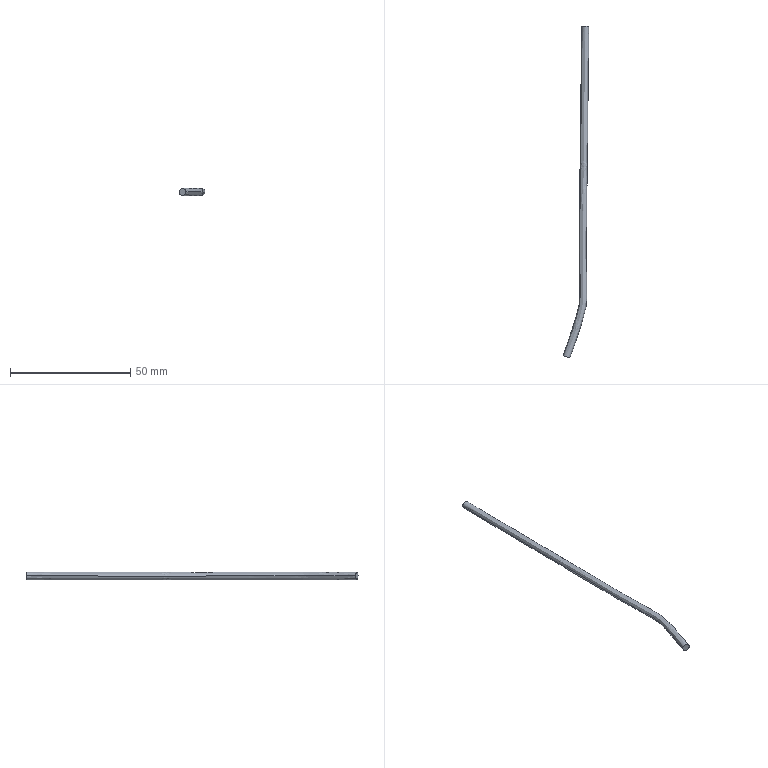Part | NX | features BREP 1 | 1 solid | 4 faces | box 10.731 x 138.267 x 3 mm | volume 970.254 mm3 | plane 2 | spline 2
STEP:
#1=CARTESIAN_POINT('',(62.397,243.449,217.465));
#2=VERTEX_POINT('',#1);
#3=CARTESIAN_POINT('',(65.397,243.411,217.465));
#4=VERTEX_POINT('',#3);
#5=CARTESIAN_POINT('',(62.397,243.449,217.465));
#6=CARTESIAN_POINT('',(62.397,243.449,217.111));
#7=CARTESIAN_POINT('',(62.665,243.445,216.338));
#8=CARTESIAN_POINT('',(63.897,243.43,215.778));
#9=CARTESIAN_POINT('',(65.129,243.415,216.338));
#10=CARTESIAN_POINT('',(65.397,243.411,217.111));
#11=CARTESIAN_POINT('',(65.397,243.411,217.465));
#12=B_SPLINE_CURVE_WITH_KNOTS('',3,(#5,#6,#7,#8,#9,#10,#11),.UNSPECIFIED.,.F.,.F.,(4,1,1,1,4),(0.,0.25,0.5,0.75,1.),.UNSPECIFIED.);
#13=EDGE_CURVE('',#2,#4,#12,.T.);
#14=ORIENTED_EDGE('',*,*,#13,.F.);
#15=CARTESIAN_POINT('',(65.397,243.411,217.465));
#16=CARTESIAN_POINT('',(65.397,243.411,217.819));
#17=CARTESIAN_POINT('',(65.129,243.415,218.592));
#18=CARTESIAN_POINT('',(63.897,243.43,219.152));
#19=CARTESIAN_POINT('',(62.665,243.445,218.592));
#20=CARTESIAN_POINT('',(62.397,243.449,217.819));
#21=CARTESIAN_POINT('',(62.397,243.449,217.465));
#22=B_SPLINE_CURVE_WITH_KNOTS('',3,(#15,#16,#17,#18,#19,#20,#21),.UNSPECIFIED.,.F.,.F.,(4,1,1,1,4),(0.,0.25,0.5,0.75,1.),.UNSPECIFIED.);
#23=EDGE_CURVE('',#4,#2,#22,.T.);
#24=ORIENTED_EDGE('',*,*,#23,.F.);
#25=EDGE_LOOP('',(#14,#24));
#26=FACE_BOUND('',#25,.T.);
#27=CARTESIAN_POINT('',(63.897,243.43,217.465));
#28=DIRECTION('',(0.01249,0.9999,0.000000006));
#29=DIRECTION('',(-0.000000489,0.,1.));
#30=AXIS2_PLACEMENT_3D('',#27,#28,#29);
#31=PLANE('',#30);
#32=ADVANCED_FACE('',(#26),#31,.T.);
#33=CARTESIAN_POINT('',(54.666,106.175,217.465));
#34=VERTEX_POINT('',#33);
#35=CARTESIAN_POINT('',(54.666,106.175,217.465));
#36=CARTESIAN_POINT('',(54.959,107.01,217.465));
#37=CARTESIAN_POINT('',(55.542,108.723,217.465));
#38=CARTESIAN_POINT('',(56.487,111.418,217.465));
#39=CARTESIAN_POINT('',(57.437,114.09,217.465));
#40=CARTESIAN_POINT('',(58.24,116.429,217.465));
#41=CARTESIAN_POINT('',(58.924,118.557,217.465));
#42=CARTESIAN_POINT('',(59.672,121.018,217.465));
#43=CARTESIAN_POINT('',(60.34,123.36,217.465));
#44=CARTESIAN_POINT('',(60.967,125.706,217.465));
#45=CARTESIAN_POINT('',(61.279,127.056,217.465));
#46=CARTESIAN_POINT('',(61.434,128.236,217.465));
#47=CARTESIAN_POINT('',(61.516,129.688,217.465));
#48=CARTESIAN_POINT('',(61.555,131.384,217.465));
#49=CARTESIAN_POINT('',(61.564,133.089,217.465));
#50=CARTESIAN_POINT('',(61.559,134.799,217.465));
#51=CARTESIAN_POINT('',(61.543,136.834,217.465));
#52=CARTESIAN_POINT('',(61.518,138.999,217.465));
#53=CARTESIAN_POINT('',(61.487,141.254,217.465));
#54=CARTESIAN_POINT('',(61.457,143.133,217.465));
#55=CARTESIAN_POINT('',(61.431,144.64,217.465));
#56=CARTESIAN_POINT('',(61.415,145.483,217.465));
#57=CARTESIAN_POINT('',(61.404,146.066,217.465));
#58=CARTESIAN_POINT('',(61.391,146.692,217.465));
#59=CARTESIAN_POINT('',(61.365,147.969,217.465));
#60=CARTESIAN_POINT('',(61.335,149.222,217.465));
#61=CARTESIAN_POINT('',(61.318,149.829,217.465));
#62=CARTESIAN_POINT('',(61.309,150.1,217.465));
#63=CARTESIAN_POINT('',(61.304,150.384,217.465));
#64=CARTESIAN_POINT('',(61.304,150.773,217.465));
#65=CARTESIAN_POINT('',(61.306,151.152,217.465));
#66=CARTESIAN_POINT('',(61.311,151.792,217.465));
#67=CARTESIAN_POINT('',(61.321,152.752,217.465));
#68=CARTESIAN_POINT('',(61.336,154.044,217.465));
#69=CARTESIAN_POINT('',(61.35,155.324,217.465));
#70=CARTESIAN_POINT('',(61.403,159.651,217.465));
#71=CARTESIAN_POINT('',(61.499,167.097,217.465));
#72=CARTESIAN_POINT('',(61.64,178.866,217.465));
#73=CARTESIAN_POINT('',(61.75,188.661,217.465));
#74=CARTESIAN_POINT('',(61.833,195.881,217.465));
#75=CARTESIAN_POINT('',(61.915,202.983,217.465));
#76=CARTESIAN_POINT('',(62.024,211.946,217.465));
#77=CARTESIAN_POINT('',(62.15,222.241,217.465));
#78=CARTESIAN_POINT('',(62.269,232.536,217.465));
#79=CARTESIAN_POINT('',(62.351,239.794,217.465));
#80=CARTESIAN_POINT('',(62.397,243.449,217.465));
#81=B_SPLINE_CURVE_WITH_KNOTS('',3,(#35,#36,#37,#38,#39,#40,#41,#42,#43,#44,#45,#46,#47,#48,#49,#50,#51,#52,#53,#54,#55,#56,#57,#58,#59,#60,#61,#62,#63,#64,#65,#66,#67,#68,#69,#70,#71,#72,#73,#74,#75,#76,#77,#78,#79,#80),.UNSPECIFIED.,.F.,.F.,(4,1,1,1,1,1,1,1,1,1,1,1,1,1,1,1,1,1,1,1,1,1,1,1,1,1,1,1,1,1,1,1,1,1,1,1,1,1,1,1,1,1,1,4),(0.,0.01988,0.03976,0.05964,0.07952,0.09481,0.1101,0.1407,0.1517,0.1628,0.1724,0.1821,0.1966,0.2112,0.2257,0.2402,0.2569,0.2736,0.2903,0.2987,0.307,0.3092,0.3114,0.3158,0.3201,0.3223,0.3245,0.3262,0.3278,0.3295,0.3311,0.3413,0.3515,0.3616,0.3718,0.4479,0.5239,0.6,0.638,0.676,0.757,0.838,0.919,1.),.UNSPECIFIED.);
#82=EDGE_CURVE('',#34,#2,#81,.T.);
#83=ORIENTED_EDGE('',*,*,#82,.T.);
#84=ORIENTED_EDGE('',*,*,#13,.T.);
#85=CARTESIAN_POINT('',(57.496,105.181,217.465));
#86=VERTEX_POINT('',#85);
#87=CARTESIAN_POINT('',(57.496,105.181,217.465));
#88=CARTESIAN_POINT('',(57.797,106.038,217.465));
#89=CARTESIAN_POINT('',(58.377,107.742,217.465));
#90=CARTESIAN_POINT('',(59.312,110.41,217.465));
#91=CARTESIAN_POINT('',(60.267,113.093,217.465));
#92=CARTESIAN_POINT('',(61.086,115.481,217.465));
#93=CARTESIAN_POINT('',(61.788,117.663,217.465));
#94=CARTESIAN_POINT('',(62.554,120.187,217.465));
#95=CARTESIAN_POINT('',(63.229,122.55,217.465));
#96=CARTESIAN_POINT('',(63.871,124.952,217.465));
#97=CARTESIAN_POINT('',(64.23,126.487,217.465));
#98=CARTESIAN_POINT('',(64.427,127.985,217.465));
#99=CARTESIAN_POINT('',(64.515,129.591,217.465));
#100=CARTESIAN_POINT('',(64.555,131.345,217.465));
#101=CARTESIAN_POINT('',(64.563,133.083,217.465));
#102=CARTESIAN_POINT('',(64.559,134.816,217.465));
#103=CARTESIAN_POINT('',(64.543,136.865,217.465));
#104=CARTESIAN_POINT('',(64.518,139.037,217.465));
#105=CARTESIAN_POINT('',(64.486,141.298,217.465));
#106=CARTESIAN_POINT('',(64.457,143.182,217.465));
#107=CARTESIAN_POINT('',(64.43,144.694,217.465));
#108=CARTESIAN_POINT('',(64.415,145.54,217.465));
#109=CARTESIAN_POINT('',(64.403,146.124,217.465));
#110=CARTESIAN_POINT('',(64.391,146.741,217.465));
#111=CARTESIAN_POINT('',(64.365,147.996,217.465));
#112=CARTESIAN_POINT('',(64.334,149.272,217.465));
#113=CARTESIAN_POINT('',(64.316,149.911,217.465));
#114=CARTESIAN_POINT('',(64.308,150.184,217.465));
#115=CARTESIAN_POINT('',(64.304,150.421,217.465));
#116=CARTESIAN_POINT('',(64.304,150.771,217.465));
#117=CARTESIAN_POINT('',(64.306,151.131,217.465));
#118=CARTESIAN_POINT('',(64.311,151.763,217.465));
#119=CARTESIAN_POINT('',(64.321,152.722,217.465));
#120=CARTESIAN_POINT('',(64.335,154.013,217.465));
#121=CARTESIAN_POINT('',(64.35,155.289,217.465));
#122=CARTESIAN_POINT('',(64.402,159.612,217.465));
#123=CARTESIAN_POINT('',(64.499,167.062,217.465));
#124=CARTESIAN_POINT('',(64.64,178.833,217.465));
#125=CARTESIAN_POINT('',(64.75,188.628,217.465));
#126=CARTESIAN_POINT('',(64.832,195.846,217.465));
#127=CARTESIAN_POINT('',(64.915,202.948,217.465));
#128=CARTESIAN_POINT('',(65.024,211.91,217.465));
#129=CARTESIAN_POINT('',(65.15,222.206,217.465));
#130=CARTESIAN_POINT('',(65.269,232.504,217.465));
#131=CARTESIAN_POINT('',(65.351,239.759,217.465));
#132=CARTESIAN_POINT('',(65.397,243.411,217.465));
#133=B_SPLINE_CURVE_WITH_KNOTS('',3,(#87,#88,#89,#90,#91,#92,#93,#94,#95,#96,#97,#98,#99,#100,#101,#102,#103,#104,#105,#106,#107,#108,#109,#110,#111,#112,#113,#114,#115,#116,#117,#118,#119,#120,#121,#122,#123,#124,#125,#126,#127,#128,#129,#130,#131,#132),.UNSPECIFIED.,.F.,.F.,(4,1,1,1,1,1,1,1,1,1,1,1,1,1,1,1,1,1,1,1,1,1,1,1,1,1,1,1,1,1,1,1,1,1,1,1,1,1,1,1,1,1,1,4),(0.,0.01988,0.03976,0.05964,0.07952,0.09481,0.1101,0.1407,0.1517,0.1628,0.1724,0.1821,0.1966,0.2112,0.2257,0.2402,0.2569,0.2736,0.2903,0.2987,0.307,0.3092,0.3114,0.3158,0.3201,0.3223,0.3245,0.3262,0.3278,0.3295,0.3311,0.3413,0.3515,0.3616,0.3718,0.4479,0.5239,0.6,0.638,0.676,0.757,0.838,0.919,1.),.UNSPECIFIED.);
#134=EDGE_CURVE('',#86,#4,#133,.T.);
#135=ORIENTED_EDGE('',*,*,#134,.F.);
#136=CARTESIAN_POINT('',(54.666,106.175,217.465));
#137=CARTESIAN_POINT('',(54.666,106.175,217.111));
#138=CARTESIAN_POINT('',(54.919,106.086,216.338));
#139=CARTESIAN_POINT('',(56.081,105.678,215.778));
#140=CARTESIAN_POINT('',(57.243,105.27,216.338));
#141=CARTESIAN_POINT('',(57.496,105.181,217.111));
#142=CARTESIAN_POINT('',(57.496,105.181,217.465));
#143=B_SPLINE_CURVE_WITH_KNOTS('',3,(#136,#137,#138,#139,#140,#141,#142),.UNSPECIFIED.,.F.,.F.,(4,1,1,1,4),(0.,0.25,0.5,0.75,1.),.UNSPECIFIED.);
#144=EDGE_CURVE('',#34,#86,#143,.T.);
#145=ORIENTED_EDGE('',*,*,#144,.F.);
#146=EDGE_LOOP('',(#83,#84,#135,#145));
#147=FACE_BOUND('',#146,.T.);
#148=CARTESIAN_POINT('',(65.397,243.411,217.465));
#149=CARTESIAN_POINT('',(65.397,243.411,217.111));
#150=CARTESIAN_POINT('',(65.129,243.415,216.338));
#151=CARTESIAN_POINT('',(63.897,243.43,215.778));
#152=CARTESIAN_POINT('',(62.665,243.445,216.338));
#153=CARTESIAN_POINT('',(62.397,243.449,217.111));
#154=CARTESIAN_POINT('',(62.397,243.449,217.465));
#155=CARTESIAN_POINT('',(65.351,239.759,217.465));
#156=CARTESIAN_POINT('',(65.351,239.759,217.111));
#157=CARTESIAN_POINT('',(65.083,239.763,216.338));
#158=CARTESIAN_POINT('',(63.851,239.777,215.778));
#159=CARTESIAN_POINT('',(62.62,239.791,216.338));
#160=CARTESIAN_POINT('',(62.351,239.794,217.111));
#161=CARTESIAN_POINT('',(62.351,239.794,217.465));
#162=CARTESIAN_POINT('',(65.269,232.504,217.465));
#163=CARTESIAN_POINT('',(65.269,232.504,217.111));
#164=CARTESIAN_POINT('',(65.001,232.506,216.338));
#165=CARTESIAN_POINT('',(63.769,232.52,215.778));
#166=CARTESIAN_POINT('',(62.537,232.533,216.338));
#167=CARTESIAN_POINT('',(62.269,232.536,217.111));
#168=CARTESIAN_POINT('',(62.269,232.536,217.465));
#169=CARTESIAN_POINT('',(65.15,222.206,217.465));
#170=CARTESIAN_POINT('',(65.15,222.206,217.111));
#171=CARTESIAN_POINT('',(64.882,222.209,216.338));
#172=CARTESIAN_POINT('',(63.65,222.223,215.778));
#173=CARTESIAN_POINT('',(62.418,222.238,216.338));
#174=CARTESIAN_POINT('',(62.15,222.241,217.111));
#175=CARTESIAN_POINT('',(62.15,222.241,217.465));
#176=CARTESIAN_POINT('',(65.024,211.91,217.465));
#177=CARTESIAN_POINT('',(65.024,211.91,217.111));
#178=CARTESIAN_POINT('',(64.756,211.913,216.338));
#179=CARTESIAN_POINT('',(63.524,211.928,215.778));
#180=CARTESIAN_POINT('',(62.292,211.943,216.338));
#181=CARTESIAN_POINT('',(62.024,211.946,217.111));
#182=CARTESIAN_POINT('',(62.024,211.946,217.465));
#183=CARTESIAN_POINT('',(64.915,202.948,217.465));
#184=CARTESIAN_POINT('',(64.915,202.948,217.111));
#185=CARTESIAN_POINT('',(64.647,202.951,216.338));
#186=CARTESIAN_POINT('',(63.415,202.965,215.778));
#187=CARTESIAN_POINT('',(62.184,202.98,216.338));
#188=CARTESIAN_POINT('',(61.915,202.983,217.111));
#189=CARTESIAN_POINT('',(61.915,202.983,217.465));
#190=CARTESIAN_POINT('',(64.832,195.846,217.465));
#191=CARTESIAN_POINT('',(64.832,195.846,217.111));
#192=CARTESIAN_POINT('',(64.564,195.85,216.338));
#193=CARTESIAN_POINT('',(63.332,195.864,215.778));
#194=CARTESIAN_POINT('',(62.101,195.878,216.338));
#195=CARTESIAN_POINT('',(61.833,195.881,217.111));
#196=CARTESIAN_POINT('',(61.833,195.881,217.465));
#197=CARTESIAN_POINT('',(64.75,188.628,217.465));
#198=CARTESIAN_POINT('',(64.75,188.628,217.111));
#199=CARTESIAN_POINT('',(64.482,188.631,216.338));
#200=CARTESIAN_POINT('',(63.25,188.644,215.778));
#201=CARTESIAN_POINT('',(62.018,188.658,216.338));
#202=CARTESIAN_POINT('',(61.75,188.661,217.111));
#203=CARTESIAN_POINT('',(61.75,188.661,217.465));
#204=CARTESIAN_POINT('',(64.64,178.833,217.465));
#205=CARTESIAN_POINT('',(64.64,178.833,217.111));
#206=CARTESIAN_POINT('',(64.371,178.836,216.338));
#207=CARTESIAN_POINT('',(63.14,178.85,215.778));
#208=CARTESIAN_POINT('',(61.908,178.863,216.338));
#209=CARTESIAN_POINT('',(61.64,178.866,217.111));
#210=CARTESIAN_POINT('',(61.64,178.866,217.465));
#211=CARTESIAN_POINT('',(64.499,167.062,217.465));
#212=CARTESIAN_POINT('',(64.499,167.062,217.111));
#213=CARTESIAN_POINT('',(64.231,167.065,216.338));
#214=CARTESIAN_POINT('',(62.999,167.08,215.778));
#215=CARTESIAN_POINT('',(61.767,167.094,216.338));
#216=CARTESIAN_POINT('',(61.499,167.097,217.111));
#217=CARTESIAN_POINT('',(61.499,167.097,217.465));
#218=CARTESIAN_POINT('',(64.402,159.612,217.465));
#219=CARTESIAN_POINT('',(64.402,159.612,217.111));
#220=CARTESIAN_POINT('',(64.134,159.615,216.338));
#221=CARTESIAN_POINT('',(62.903,159.632,215.778));
#222=CARTESIAN_POINT('',(61.671,159.648,216.338));
#223=CARTESIAN_POINT('',(61.403,159.651,217.111));
#224=CARTESIAN_POINT('',(61.403,159.651,217.465));
#225=CARTESIAN_POINT('',(64.35,155.289,217.465));
#226=CARTESIAN_POINT('',(64.35,155.289,217.111));
#227=CARTESIAN_POINT('',(64.082,155.292,216.338));
#228=CARTESIAN_POINT('',(62.85,155.307,215.778));
#229=CARTESIAN_POINT('',(61.618,155.321,216.338));
#230=CARTESIAN_POINT('',(61.35,155.324,217.111));
#231=CARTESIAN_POINT('',(61.35,155.324,217.465));
#232=CARTESIAN_POINT('',(64.335,154.013,217.465));
#233=CARTESIAN_POINT('',(64.335,154.013,217.111));
#234=CARTESIAN_POINT('',(64.067,154.015,216.338));
#235=CARTESIAN_POINT('',(62.835,154.028,215.778));
#236=CARTESIAN_POINT('',(61.604,154.041,216.338));
#237=CARTESIAN_POINT('',(61.336,154.044,217.111));
#238=CARTESIAN_POINT('',(61.336,154.044,217.465));
#239=CARTESIAN_POINT('',(64.321,152.722,217.465));
#240=CARTESIAN_POINT('',(64.321,152.722,217.111));
#241=CARTESIAN_POINT('',(64.053,152.724,216.338));
#242=CARTESIAN_POINT('',(62.821,152.737,215.778));
#243=CARTESIAN_POINT('',(61.589,152.749,216.338));
#244=CARTESIAN_POINT('',(61.321,152.752,217.111));
#245=CARTESIAN_POINT('',(61.321,152.752,217.465));
#246=CARTESIAN_POINT('',(64.311,151.763,217.465));
#247=CARTESIAN_POINT('',(64.311,151.763,217.111));
#248=CARTESIAN_POINT('',(64.043,151.766,216.338));
#249=CARTESIAN_POINT('',(62.811,151.778,215.778));
#250=CARTESIAN_POINT('',(61.579,151.79,216.338));
#251=CARTESIAN_POINT('',(61.311,151.792,217.111));
#252=CARTESIAN_POINT('',(61.311,151.792,217.465));
#253=CARTESIAN_POINT('',(64.306,151.131,217.465));
#254=CARTESIAN_POINT('',(64.306,151.131,217.111));
#255=CARTESIAN_POINT('',(64.038,151.133,216.338));
#256=CARTESIAN_POINT('',(62.806,151.141,215.778));
#257=CARTESIAN_POINT('',(61.574,151.15,216.338));
#258=CARTESIAN_POINT('',(61.306,151.152,217.111));
#259=CARTESIAN_POINT('',(61.306,151.152,217.465));
#260=CARTESIAN_POINT('',(64.304,150.771,217.465));
#261=CARTESIAN_POINT('',(64.304,150.771,217.111));
#262=CARTESIAN_POINT('',(64.036,150.771,216.338));
#263=CARTESIAN_POINT('',(62.804,150.772,215.778));
#264=CARTESIAN_POINT('',(61.572,150.772,216.338));
#265=CARTESIAN_POINT('',(61.304,150.773,217.111));
#266=CARTESIAN_POINT('',(61.304,150.773,217.465));
#267=CARTESIAN_POINT('',(64.304,150.421,217.465));
#268=CARTESIAN_POINT('',(64.304,150.421,217.111));
#269=CARTESIAN_POINT('',(64.036,150.417,216.338));
#270=CARTESIAN_POINT('',(62.804,150.402,215.778));
#271=CARTESIAN_POINT('',(61.572,150.388,216.338));
#272=CARTESIAN_POINT('',(61.304,150.384,217.111));
#273=CARTESIAN_POINT('',(61.304,150.384,217.465));
#274=CARTESIAN_POINT('',(64.308,150.184,217.465));
#275=CARTESIAN_POINT('',(64.308,150.184,217.111));
#276=CARTESIAN_POINT('',(64.04,150.177,216.338));
#277=CARTESIAN_POINT('',(62.809,150.142,215.778));
#278=CARTESIAN_POINT('',(61.578,150.108,216.338));
#279=CARTESIAN_POINT('',(61.309,150.1,217.111));
#280=CARTESIAN_POINT('',(61.309,150.1,217.465));
#281=CARTESIAN_POINT('',(64.316,149.911,217.465));
#282=CARTESIAN_POINT('',(64.316,149.911,217.111));
#283=CARTESIAN_POINT('',(64.048,149.903,216.338));
#284=CARTESIAN_POINT('',(62.817,149.87,215.778));
#285=CARTESIAN_POINT('',(61.586,149.836,216.338));
#286=CARTESIAN_POINT('',(61.318,149.829,217.111));
#287=CARTESIAN_POINT('',(61.318,149.829,217.465));
#288=CARTESIAN_POINT('',(64.334,149.272,217.465));
#289=CARTESIAN_POINT('',(64.334,149.272,217.111));
#290=CARTESIAN_POINT('',(64.066,149.267,216.338));
#291=CARTESIAN_POINT('',(62.834,149.247,215.778));
#292=CARTESIAN_POINT('',(61.603,149.227,216.338));
#293=CARTESIAN_POINT('',(61.335,149.222,217.111));
#294=CARTESIAN_POINT('',(61.335,149.222,217.465));
#295=CARTESIAN_POINT('',(64.365,147.996,217.465));
#296=CARTESIAN_POINT('',(64.365,147.996,217.111));
#297=CARTESIAN_POINT('',(64.096,147.993,216.338));
#298=CARTESIAN_POINT('',(62.865,147.982,215.778));
#299=CARTESIAN_POINT('',(61.633,147.972,216.338));
#300=CARTESIAN_POINT('',(61.365,147.969,217.111));
#301=CARTESIAN_POINT('',(61.365,147.969,217.465));
#302=CARTESIAN_POINT('',(64.391,146.741,217.465));
#303=CARTESIAN_POINT('',(64.391,146.741,217.111));
#304=CARTESIAN_POINT('',(64.123,146.737,216.338));
#305=CARTESIAN_POINT('',(62.891,146.717,215.778));
#306=CARTESIAN_POINT('',(61.66,146.697,216.338));
#307=CARTESIAN_POINT('',(61.391,146.692,217.111));
#308=CARTESIAN_POINT('',(61.391,146.692,217.465));
#309=CARTESIAN_POINT('',(64.403,146.124,217.465));
#310=CARTESIAN_POINT('',(64.403,146.124,217.111));
#311=CARTESIAN_POINT('',(64.135,146.119,216.338));
#312=CARTESIAN_POINT('',(62.904,146.095,215.778));
#313=CARTESIAN_POINT('',(61.672,146.071,216.338));
#314=CARTESIAN_POINT('',(61.404,146.066,217.111));
#315=CARTESIAN_POINT('',(61.404,146.066,217.465));
#316=CARTESIAN_POINT('',(64.415,145.54,217.465));
#317=CARTESIAN_POINT('',(64.415,145.54,217.111));
#318=CARTESIAN_POINT('',(64.146,145.535,216.338));
#319=CARTESIAN_POINT('',(62.915,145.511,215.778));
#320=CARTESIAN_POINT('',(61.683,145.488,216.338));
#321=CARTESIAN_POINT('',(61.415,145.483,217.111));
#322=CARTESIAN_POINT('',(61.415,145.483,217.465));
#323=CARTESIAN_POINT('',(64.43,144.694,217.465));
#324=CARTESIAN_POINT('',(64.43,144.694,217.111));
#325=CARTESIAN_POINT('',(64.162,144.689,216.338));
#326=CARTESIAN_POINT('',(62.931,144.667,215.778));
#327=CARTESIAN_POINT('',(61.699,144.645,216.338));
#328=CARTESIAN_POINT('',(61.431,144.64,217.111));
#329=CARTESIAN_POINT('',(61.431,144.64,217.465));
#330=CARTESIAN_POINT('',(64.457,143.182,217.465));
#331=CARTESIAN_POINT('',(64.457,143.182,217.111));
#332=CARTESIAN_POINT('',(64.188,143.178,216.338));
#333=CARTESIAN_POINT('',(62.957,143.158,215.778));
#334=CARTESIAN_POINT('',(61.725,143.137,216.338));
#335=CARTESIAN_POINT('',(61.457,143.133,217.111));
#336=CARTESIAN_POINT('',(61.457,143.133,217.465));
#337=CARTESIAN_POINT('',(64.486,141.298,217.465));
#338=CARTESIAN_POINT('',(64.486,141.298,217.111));
#339=CARTESIAN_POINT('',(64.218,141.294,216.338));
#340=CARTESIAN_POINT('',(62.986,141.276,215.778));
#341=CARTESIAN_POINT('',(61.755,141.258,216.338));
#342=CARTESIAN_POINT('',(61.487,141.254,217.111));
#343=CARTESIAN_POINT('',(61.487,141.254,217.465));
#344=CARTESIAN_POINT('',(64.518,139.037,217.465));
#345=CARTESIAN_POINT('',(64.518,139.037,217.111));
#346=CARTESIAN_POINT('',(64.249,139.033,216.338));
#347=CARTESIAN_POINT('',(63.018,139.018,215.778));
#348=CARTESIAN_POINT('',(61.786,139.002,216.338));
#349=CARTESIAN_POINT('',(61.518,138.999,217.111));
#350=CARTESIAN_POINT('',(61.518,138.999,217.465));
#351=CARTESIAN_POINT('',(64.543,136.865,217.465));
#352=CARTESIAN_POINT('',(64.543,136.865,217.111));
#353=CARTESIAN_POINT('',(64.274,136.862,216.338));
#354=CARTESIAN_POINT('',(63.043,136.849,215.778));
#355=CARTESIAN_POINT('',(61.811,136.837,216.338));
#356=CARTESIAN_POINT('',(61.543,136.834,217.111));
#357=CARTESIAN_POINT('',(61.543,136.834,217.465));
#358=CARTESIAN_POINT('',(64.559,134.816,217.465));
#359=CARTESIAN_POINT('',(64.559,134.816,217.111));
#360=CARTESIAN_POINT('',(64.291,134.814,216.338));
#361=CARTESIAN_POINT('',(63.059,134.808,215.778));
#362=CARTESIAN_POINT('',(61.827,134.801,216.338));
#363=CARTESIAN_POINT('',(61.559,134.799,217.111));
#364=CARTESIAN_POINT('',(61.559,134.799,217.465));
#365=CARTESIAN_POINT('',(64.563,133.083,217.465));
#366=CARTESIAN_POINT('',(64.563,133.083,217.111));
#367=CARTESIAN_POINT('',(64.295,133.084,216.338));
#368=CARTESIAN_POINT('',(63.064,133.086,215.778));
#369=CARTESIAN_POINT('',(61.832,133.089,216.338));
#370=CARTESIAN_POINT('',(61.564,133.089,217.111));
#371=CARTESIAN_POINT('',(61.564,133.089,217.465));
#372=CARTESIAN_POINT('',(64.555,131.345,217.465));
#373=CARTESIAN_POINT('',(64.555,131.345,217.111));
#374=CARTESIAN_POINT('',(64.287,131.348,216.338));
#375=CARTESIAN_POINT('',(63.055,131.364,215.778));
#376=CARTESIAN_POINT('',(61.823,131.381,216.338));
#377=CARTESIAN_POINT('',(61.555,131.384,217.111));
#378=CARTESIAN_POINT('',(61.555,131.384,217.465));
#379=CARTESIAN_POINT('',(64.515,129.591,217.465));
#380=CARTESIAN_POINT('',(64.515,129.591,217.111));
#381=CARTESIAN_POINT('',(64.246,129.599,216.338));
#382=CARTESIAN_POINT('',(63.015,129.639,215.778));
#383=CARTESIAN_POINT('',(61.784,129.679,216.338));
#384=CARTESIAN_POINT('',(61.516,129.688,217.111));
#385=CARTESIAN_POINT('',(61.516,129.688,217.465));
#386=CARTESIAN_POINT('',(64.427,127.985,217.465));
#387=CARTESIAN_POINT('',(64.427,127.985,217.111));
#388=CARTESIAN_POINT('',(64.159,128.008,216.338));
#389=CARTESIAN_POINT('',(62.93,128.111,215.778));
#390=CARTESIAN_POINT('',(61.701,128.214,216.338));
#391=CARTESIAN_POINT('',(61.434,128.236,217.111));
#392=CARTESIAN_POINT('',(61.434,128.236,217.465));
#393=CARTESIAN_POINT('',(64.23,126.487,217.465));
#394=CARTESIAN_POINT('',(64.23,126.487,217.111));
#395=CARTESIAN_POINT('',(63.966,126.538,216.338));
#396=CARTESIAN_POINT('',(62.754,126.771,215.778));
#397=CARTESIAN_POINT('',(61.543,127.005,216.338));
#398=CARTESIAN_POINT('',(61.279,127.056,217.111));
#399=CARTESIAN_POINT('',(61.279,127.056,217.465));
#400=CARTESIAN_POINT('',(63.871,124.952,217.465));
#401=CARTESIAN_POINT('',(63.871,124.952,217.111));
#402=CARTESIAN_POINT('',(63.611,125.019,216.338));
#403=CARTESIAN_POINT('',(62.419,125.329,215.778));
#404=CARTESIAN_POINT('',(61.226,125.638,216.338));
#405=CARTESIAN_POINT('',(60.967,125.706,217.111));
#406=CARTESIAN_POINT('',(60.967,125.706,217.465));
#407=CARTESIAN_POINT('',(63.229,122.55,217.465));
#408=CARTESIAN_POINT('',(63.229,122.55,217.111));
#409=CARTESIAN_POINT('',(62.97,122.622,216.338));
#410=CARTESIAN_POINT('',(61.784,122.955,215.778));
#411=CARTESIAN_POINT('',(60.599,123.288,216.338));
#412=CARTESIAN_POINT('',(60.34,123.36,217.111));
#413=CARTESIAN_POINT('',(60.34,123.36,217.465));
#414=CARTESIAN_POINT('',(62.554,120.187,217.465));
#415=CARTESIAN_POINT('',(62.554,120.187,217.111));
#416=CARTESIAN_POINT('',(62.297,120.261,216.338));
#417=CARTESIAN_POINT('',(61.113,120.603,215.778));
#418=CARTESIAN_POINT('',(59.93,120.944,216.338));
#419=CARTESIAN_POINT('',(59.672,121.018,217.111));
#420=CARTESIAN_POINT('',(59.672,121.018,217.465));
#421=CARTESIAN_POINT('',(61.788,117.663,217.465));
#422=CARTESIAN_POINT('',(61.788,117.663,217.111));
#423=CARTESIAN_POINT('',(61.532,117.742,216.338));
#424=CARTESIAN_POINT('',(60.356,118.11,215.778));
#425=CARTESIAN_POINT('',(59.18,118.477,216.338));
#426=CARTESIAN_POINT('',(58.924,118.557,217.111));
#427=CARTESIAN_POINT('',(58.924,118.557,217.465));
#428=CARTESIAN_POINT('',(61.086,115.481,217.465));
#429=CARTESIAN_POINT('',(61.086,115.481,217.111));
#430=CARTESIAN_POINT('',(60.832,115.566,216.338));
#431=CARTESIAN_POINT('',(59.663,115.955,215.778));
#432=CARTESIAN_POINT('',(58.494,116.345,216.338));
#433=CARTESIAN_POINT('',(58.24,116.429,217.111));
#434=CARTESIAN_POINT('',(58.24,116.429,217.465));
#435=CARTESIAN_POINT('',(60.267,113.093,217.465));
#436=CARTESIAN_POINT('',(60.267,113.093,217.111));
#437=CARTESIAN_POINT('',(60.014,113.182,216.338));
#438=CARTESIAN_POINT('',(58.852,113.591,215.778));
#439=CARTESIAN_POINT('',(57.69,114.001,216.338));
#440=CARTESIAN_POINT('',(57.437,114.09,217.111));
#441=CARTESIAN_POINT('',(57.437,114.09,217.465));
#442=CARTESIAN_POINT('',(59.312,110.41,217.465));
#443=CARTESIAN_POINT('',(59.312,110.41,217.111));
#444=CARTESIAN_POINT('',(59.059,110.5,216.338));
#445=CARTESIAN_POINT('',(57.899,110.914,215.778));
#446=CARTESIAN_POINT('',(56.739,111.328,216.338));
#447=CARTESIAN_POINT('',(56.487,111.418,217.111));
#448=CARTESIAN_POINT('',(56.487,111.418,217.465));
#449=CARTESIAN_POINT('',(58.377,107.742,217.465));
#450=CARTESIAN_POINT('',(58.377,107.742,217.111));
#451=CARTESIAN_POINT('',(58.124,107.83,216.338));
#452=CARTESIAN_POINT('',(56.96,108.232,215.778));
#453=CARTESIAN_POINT('',(55.796,108.635,216.338));
#454=CARTESIAN_POINT('',(55.542,108.723,217.111));
#455=CARTESIAN_POINT('',(55.542,108.723,217.465));
#456=CARTESIAN_POINT('',(57.797,106.038,217.465));
#457=CARTESIAN_POINT('',(57.797,106.038,217.111));
#458=CARTESIAN_POINT('',(57.543,106.125,216.338));
#459=CARTESIAN_POINT('',(56.378,106.524,215.778));
#460=CARTESIAN_POINT('',(55.213,106.923,216.338));
#461=CARTESIAN_POINT('',(54.959,107.01,217.111));
#462=CARTESIAN_POINT('',(54.959,107.01,217.465));
#463=CARTESIAN_POINT('',(57.496,105.181,217.465));
#464=CARTESIAN_POINT('',(57.496,105.181,217.111));
#465=CARTESIAN_POINT('',(57.243,105.27,216.338));
#466=CARTESIAN_POINT('',(56.081,105.678,215.778));
#467=CARTESIAN_POINT('',(54.919,106.086,216.338));
#468=CARTESIAN_POINT('',(54.666,106.175,217.111));
#469=CARTESIAN_POINT('',(54.666,106.175,217.465));
#470=B_SPLINE_SURFACE_WITH_KNOTS('',3,3,((#148,#149,#150,#151,#152,#153,#154),(#155,#156,#157,#158,#159,#160,#161),(#162,#163,#164,#165,#166,#167,#168),(#169,#170,#171,#172,#173,#174,#175),(#176,#177,#178,#179,#180,#181,#182),(#183,#184,#185,#186,#187,#188,#189),(#190,#191,#192,#193,#194,#195,#196),(#197,#198,#199,#200,#201,#202,#203),(#204,#205,#206,#207,#208,#209,#210),(#211,#212,#213,#214,#215,#216,#217),(#218,#219,#220,#221,#222,#223,#224),(#225,#226,#227,#228,#229,#230,#231),(#232,#233,#234,#235,#236,#237,#238),(#239,#240,#241,#242,#243,#244,#245),(#246,#247,#248,#249,#250,#251,#252),(#253,#254,#255,#256,#257,#258,#259),(#260,#261,#262,#263,#264,#265,#266),(#267,#268,#269,#270,#271,#272,#273),(#274,#275,#276,#277,#278,#279,#280),(#281,#282,#283,#284,#285,#286,#287),(#288,#289,#290,#291,#292,#293,#294),(#295,#296,#297,#298,#299,#300,#301),(#302,#303,#304,#305,#306,#307,#308),(#309,#310,#311,#312,#313,#314,#315),(#316,#317,#318,#319,#320,#321,#322),(#323,#324,#325,#326,#327,#328,#329),(#330,#331,#332,#333,#334,#335,#336),(#337,#338,#339,#340,#341,#342,#343),(#344,#345,#346,#347,#348,#349,#350),(#351,#352,#353,#354,#355,#356,#357),(#358,#359,#360,#361,#362,#363,#364),(#365,#366,#367,#368,#369,#370,#371),(#372,#373,#374,#375,#376,#377,#378),(#379,#380,#381,#382,#383,#384,#385),(#386,#387,#388,#389,#390,#391,#392),(#393,#394,#395,#396,#397,#398,#399),(#400,#401,#402,#403,#404,#405,#406),(#407,#408,#409,#410,#411,#412,#413),(#414,#415,#416,#417,#418,#419,#420),(#421,#422,#423,#424,#425,#426,#427),(#428,#429,#430,#431,#432,#433,#434),(#435,#436,#437,#438,#439,#440,#441),(#442,#443,#444,#445,#446,#447,#448),(#449,#450,#451,#452,#453,#454,#455),(#456,#457,#458,#459,#460,#461,#462),(#463,#464,#465,#466,#467,#468,#469)),.UNSPECIFIED.,.F.,.F.,.F.,(4,1,1,1,1,1,1,1,1,1,1,1,1,1,1,1,1,1,1,1,1,1,1,1,1,1,1,1,1,1,1,1,1,1,1,1,1,1,1,1,1,1,1,4),(4,1,1,1,4),(0.009994,0.08937,0.1687,0.2481,0.3275,0.3648,0.402,0.4766,0.5511,0.6256,0.6356,0.6456,0.6555,0.6655,0.6671,0.6687,0.6704,0.672,0.6741,0.6763,0.6805,0.6848,0.687,0.6891,0.6973,0.7055,0.7218,0.7382,0.7546,0.7688,0.783,0.7973,0.8115,0.821,0.8305,0.8413,0.8521,0.8821,0.8971,0.912,0.9315,0.951,0.9705,0.99),(0.02108,0.2606,0.5002,0.7397,0.9793),.UNSPECIFIED.);
#471=ADVANCED_FACE('',(#147),#470,.T.);
#472=ORIENTED_EDGE('',*,*,#134,.T.);
#473=ORIENTED_EDGE('',*,*,#23,.T.);
#474=ORIENTED_EDGE('',*,*,#82,.F.);
#475=CARTESIAN_POINT('',(57.496,105.181,217.465));
#476=CARTESIAN_POINT('',(57.496,105.181,217.819));
#477=CARTESIAN_POINT('',(57.243,105.27,218.592));
#478=CARTESIAN_POINT('',(56.081,105.678,219.152));
#479=CARTESIAN_POINT('',(54.919,106.086,218.592));
#480=CARTESIAN_POINT('',(54.666,106.175,217.819));
#481=CARTESIAN_POINT('',(54.666,106.175,217.465));
#482=B_SPLINE_CURVE_WITH_KNOTS('',3,(#475,#476,#477,#478,#479,#480,#481),.UNSPECIFIED.,.F.,.F.,(4,1,1,1,4),(0.,0.25,0.5,0.75,1.),.UNSPECIFIED.);
#483=EDGE_CURVE('',#86,#34,#482,.T.);
#484=ORIENTED_EDGE('',*,*,#483,.F.);
#485=EDGE_LOOP('',(#472,#473,#474,#484));
#486=FACE_BOUND('',#485,.T.);
#487=CARTESIAN_POINT('',(62.397,243.449,217.465));
#488=CARTESIAN_POINT('',(62.397,243.449,217.819));
#489=CARTESIAN_POINT('',(62.665,243.445,218.592));
#490=CARTESIAN_POINT('',(63.897,243.43,219.152));
#491=CARTESIAN_POINT('',(65.129,243.415,218.592));
#492=CARTESIAN_POINT('',(65.397,243.411,217.819));
#493=CARTESIAN_POINT('',(65.397,243.411,217.465));
#494=CARTESIAN_POINT('',(62.351,239.794,217.465));
#495=CARTESIAN_POINT('',(62.351,239.794,217.819));
#496=CARTESIAN_POINT('',(62.62,239.791,218.592));
#497=CARTESIAN_POINT('',(63.851,239.777,219.152));
#498=CARTESIAN_POINT('',(65.083,239.763,218.592));
#499=CARTESIAN_POINT('',(65.351,239.759,217.819));
#500=CARTESIAN_POINT('',(65.351,239.759,217.465));
#501=CARTESIAN_POINT('',(62.269,232.536,217.465));
#502=CARTESIAN_POINT('',(62.269,232.536,217.819));
#503=CARTESIAN_POINT('',(62.537,232.533,218.592));
#504=CARTESIAN_POINT('',(63.769,232.52,219.152));
#505=CARTESIAN_POINT('',(65.001,232.506,218.592));
#506=CARTESIAN_POINT('',(65.269,232.504,217.819));
#507=CARTESIAN_POINT('',(65.269,232.504,217.465));
#508=CARTESIAN_POINT('',(62.15,222.241,217.465));
#509=CARTESIAN_POINT('',(62.15,222.241,217.819));
#510=CARTESIAN_POINT('',(62.418,222.238,218.592));
#511=CARTESIAN_POINT('',(63.65,222.223,219.152));
#512=CARTESIAN_POINT('',(64.882,222.209,218.592));
#513=CARTESIAN_POINT('',(65.15,222.206,217.819));
#514=CARTESIAN_POINT('',(65.15,222.206,217.465));
#515=CARTESIAN_POINT('',(62.024,211.946,217.465));
#516=CARTESIAN_POINT('',(62.024,211.946,217.819));
#517=CARTESIAN_POINT('',(62.292,211.943,218.592));
#518=CARTESIAN_POINT('',(63.524,211.928,219.152));
#519=CARTESIAN_POINT('',(64.756,211.913,218.592));
#520=CARTESIAN_POINT('',(65.024,211.91,217.819));
#521=CARTESIAN_POINT('',(65.024,211.91,217.465));
#522=CARTESIAN_POINT('',(61.915,202.983,217.465));
#523=CARTESIAN_POINT('',(61.915,202.983,217.819));
#524=CARTESIAN_POINT('',(62.184,202.98,218.592));
#525=CARTESIAN_POINT('',(63.415,202.965,219.152));
#526=CARTESIAN_POINT('',(64.647,202.951,218.592));
#527=CARTESIAN_POINT('',(64.915,202.948,217.819));
#528=CARTESIAN_POINT('',(64.915,202.948,217.465));
#529=CARTESIAN_POINT('',(61.833,195.881,217.465));
#530=CARTESIAN_POINT('',(61.833,195.881,217.819));
#531=CARTESIAN_POINT('',(62.101,195.878,218.592));
#532=CARTESIAN_POINT('',(63.332,195.864,219.152));
#533=CARTESIAN_POINT('',(64.564,195.85,218.592));
#534=CARTESIAN_POINT('',(64.832,195.846,217.819));
#535=CARTESIAN_POINT('',(64.832,195.846,217.465));
#536=CARTESIAN_POINT('',(61.75,188.661,217.465));
#537=CARTESIAN_POINT('',(61.75,188.661,217.819));
#538=CARTESIAN_POINT('',(62.018,188.658,218.592));
#539=CARTESIAN_POINT('',(63.25,188.644,219.152));
#540=CARTESIAN_POINT('',(64.482,188.631,218.592));
#541=CARTESIAN_POINT('',(64.75,188.628,217.819));
#542=CARTESIAN_POINT('',(64.75,188.628,217.465));
#543=CARTESIAN_POINT('',(61.64,178.866,217.465));
#544=CARTESIAN_POINT('',(61.64,178.866,217.819));
#545=CARTESIAN_POINT('',(61.908,178.863,218.592));
#546=CARTESIAN_POINT('',(63.14,178.85,219.152));
#547=CARTESIAN_POINT('',(64.371,178.836,218.592));
#548=CARTESIAN_POINT('',(64.64,178.833,217.819));
#549=CARTESIAN_POINT('',(64.64,178.833,217.465));
#550=CARTESIAN_POINT('',(61.499,167.097,217.465));
#551=CARTESIAN_POINT('',(61.499,167.097,217.819));
#552=CARTESIAN_POINT('',(61.767,167.094,218.592));
#553=CARTESIAN_POINT('',(62.999,167.08,219.152));
#554=CARTESIAN_POINT('',(64.231,167.065,218.592));
#555=CARTESIAN_POINT('',(64.499,167.062,217.819));
#556=CARTESIAN_POINT('',(64.499,167.062,217.465));
#557=CARTESIAN_POINT('',(61.403,159.651,217.465));
#558=CARTESIAN_POINT('',(61.403,159.651,217.819));
#559=CARTESIAN_POINT('',(61.671,159.648,218.592));
#560=CARTESIAN_POINT('',(62.903,159.632,219.152));
#561=CARTESIAN_POINT('',(64.134,159.615,218.592));
#562=CARTESIAN_POINT('',(64.402,159.612,217.819));
#563=CARTESIAN_POINT('',(64.402,159.612,217.465));
#564=CARTESIAN_POINT('',(61.35,155.324,217.465));
#565=CARTESIAN_POINT('',(61.35,155.324,217.819));
#566=CARTESIAN_POINT('',(61.618,155.321,218.592));
#567=CARTESIAN_POINT('',(62.85,155.307,219.152));
#568=CARTESIAN_POINT('',(64.082,155.292,218.592));
#569=CARTESIAN_POINT('',(64.35,155.289,217.819));
#570=CARTESIAN_POINT('',(64.35,155.289,217.465));
#571=CARTESIAN_POINT('',(61.336,154.044,217.465));
#572=CARTESIAN_POINT('',(61.336,154.044,217.819));
#573=CARTESIAN_POINT('',(61.604,154.041,218.592));
#574=CARTESIAN_POINT('',(62.835,154.028,219.152));
#575=CARTESIAN_POINT('',(64.067,154.015,218.592));
#576=CARTESIAN_POINT('',(64.335,154.013,217.819));
#577=CARTESIAN_POINT('',(64.335,154.013,217.465));
#578=CARTESIAN_POINT('',(61.321,152.752,217.465));
#579=CARTESIAN_POINT('',(61.321,152.752,217.819));
#580=CARTESIAN_POINT('',(61.589,152.749,218.592));
#581=CARTESIAN_POINT('',(62.821,152.737,219.152));
#582=CARTESIAN_POINT('',(64.053,152.724,218.592));
#583=CARTESIAN_POINT('',(64.321,152.722,217.819));
#584=CARTESIAN_POINT('',(64.321,152.722,217.465));
#585=CARTESIAN_POINT('',(61.311,151.792,217.465));
#586=CARTESIAN_POINT('',(61.311,151.792,217.819));
#587=CARTESIAN_POINT('',(61.579,151.79,218.592));
#588=CARTESIAN_POINT('',(62.811,151.778,219.152));
#589=CARTESIAN_POINT('',(64.043,151.766,218.592));
#590=CARTESIAN_POINT('',(64.311,151.763,217.819));
#591=CARTESIAN_POINT('',(64.311,151.763,217.465));
#592=CARTESIAN_POINT('',(61.306,151.152,217.465));
#593=CARTESIAN_POINT('',(61.306,151.152,217.819));
#594=CARTESIAN_POINT('',(61.574,151.15,218.592));
#595=CARTESIAN_POINT('',(62.806,151.141,219.152));
#596=CARTESIAN_POINT('',(64.038,151.133,218.592));
#597=CARTESIAN_POINT('',(64.306,151.131,217.819));
#598=CARTESIAN_POINT('',(64.306,151.131,217.465));
#599=CARTESIAN_POINT('',(61.304,150.773,217.465));
#600=CARTESIAN_POINT('',(61.304,150.773,217.819));
#601=CARTESIAN_POINT('',(61.572,150.772,218.592));
#602=CARTESIAN_POINT('',(62.804,150.772,219.152));
#603=CARTESIAN_POINT('',(64.036,150.771,218.592));
#604=CARTESIAN_POINT('',(64.304,150.771,217.819));
#605=CARTESIAN_POINT('',(64.304,150.771,217.465));
#606=CARTESIAN_POINT('',(61.304,150.384,217.465));
#607=CARTESIAN_POINT('',(61.304,150.384,217.819));
#608=CARTESIAN_POINT('',(61.572,150.388,218.592));
#609=CARTESIAN_POINT('',(62.804,150.402,219.152));
#610=CARTESIAN_POINT('',(64.036,150.417,218.592));
#611=CARTESIAN_POINT('',(64.304,150.421,217.819));
#612=CARTESIAN_POINT('',(64.304,150.421,217.465));
#613=CARTESIAN_POINT('',(61.309,150.1,217.465));
#614=CARTESIAN_POINT('',(61.309,150.1,217.819));
#615=CARTESIAN_POINT('',(61.578,150.108,218.592));
#616=CARTESIAN_POINT('',(62.809,150.142,219.152));
#617=CARTESIAN_POINT('',(64.04,150.177,218.592));
#618=CARTESIAN_POINT('',(64.308,150.184,217.819));
#619=CARTESIAN_POINT('',(64.308,150.184,217.465));
#620=CARTESIAN_POINT('',(61.318,149.829,217.465));
#621=CARTESIAN_POINT('',(61.318,149.829,217.819));
#622=CARTESIAN_POINT('',(61.586,149.836,218.592));
#623=CARTESIAN_POINT('',(62.817,149.87,219.152));
#624=CARTESIAN_POINT('',(64.048,149.903,218.592));
#625=CARTESIAN_POINT('',(64.316,149.911,217.819));
#626=CARTESIAN_POINT('',(64.316,149.911,217.465));
#627=CARTESIAN_POINT('',(61.335,149.222,217.465));
#628=CARTESIAN_POINT('',(61.335,149.222,217.819));
#629=CARTESIAN_POINT('',(61.603,149.227,218.592));
#630=CARTESIAN_POINT('',(62.834,149.247,219.152));
#631=CARTESIAN_POINT('',(64.066,149.267,218.592));
#632=CARTESIAN_POINT('',(64.334,149.272,217.819));
#633=CARTESIAN_POINT('',(64.334,149.272,217.465));
#634=CARTESIAN_POINT('',(61.365,147.969,217.465));
#635=CARTESIAN_POINT('',(61.365,147.969,217.819));
#636=CARTESIAN_POINT('',(61.633,147.972,218.592));
#637=CARTESIAN_POINT('',(62.865,147.982,219.152));
#638=CARTESIAN_POINT('',(64.096,147.993,218.592));
#639=CARTESIAN_POINT('',(64.365,147.996,217.819));
#640=CARTESIAN_POINT('',(64.365,147.996,217.465));
#641=CARTESIAN_POINT('',(61.391,146.692,217.465));
#642=CARTESIAN_POINT('',(61.391,146.692,217.819));
#643=CARTESIAN_POINT('',(61.66,146.697,218.592));
#644=CARTESIAN_POINT('',(62.891,146.717,219.152));
#645=CARTESIAN_POINT('',(64.123,146.737,218.592));
#646=CARTESIAN_POINT('',(64.391,146.741,217.819));
#647=CARTESIAN_POINT('',(64.391,146.741,217.465));
#648=CARTESIAN_POINT('',(61.404,146.066,217.465));
#649=CARTESIAN_POINT('',(61.404,146.066,217.819));
#650=CARTESIAN_POINT('',(61.672,146.071,218.592));
#651=CARTESIAN_POINT('',(62.904,146.095,219.152));
#652=CARTESIAN_POINT('',(64.135,146.119,218.592));
#653=CARTESIAN_POINT('',(64.403,146.124,217.819));
#654=CARTESIAN_POINT('',(64.403,146.124,217.465));
#655=CARTESIAN_POINT('',(61.415,145.483,217.465));
#656=CARTESIAN_POINT('',(61.415,145.483,217.819));
#657=CARTESIAN_POINT('',(61.683,145.488,218.592));
#658=CARTESIAN_POINT('',(62.915,145.511,219.152));
#659=CARTESIAN_POINT('',(64.146,145.535,218.592));
#660=CARTESIAN_POINT('',(64.415,145.54,217.819));
#661=CARTESIAN_POINT('',(64.415,145.54,217.465));
#662=CARTESIAN_POINT('',(61.431,144.64,217.465));
#663=CARTESIAN_POINT('',(61.431,144.64,217.819));
#664=CARTESIAN_POINT('',(61.699,144.645,218.592));
#665=CARTESIAN_POINT('',(62.931,144.667,219.152));
#666=CARTESIAN_POINT('',(64.162,144.689,218.592));
#667=CARTESIAN_POINT('',(64.43,144.694,217.819));
#668=CARTESIAN_POINT('',(64.43,144.694,217.465));
#669=CARTESIAN_POINT('',(61.457,143.133,217.465));
#670=CARTESIAN_POINT('',(61.457,143.133,217.819));
#671=CARTESIAN_POINT('',(61.725,143.137,218.592));
#672=CARTESIAN_POINT('',(62.957,143.158,219.152));
#673=CARTESIAN_POINT('',(64.188,143.178,218.592));
#674=CARTESIAN_POINT('',(64.457,143.182,217.819));
#675=CARTESIAN_POINT('',(64.457,143.182,217.465));
#676=CARTESIAN_POINT('',(61.487,141.254,217.465));
#677=CARTESIAN_POINT('',(61.487,141.254,217.819));
#678=CARTESIAN_POINT('',(61.755,141.258,218.592));
#679=CARTESIAN_POINT('',(62.986,141.276,219.152));
#680=CARTESIAN_POINT('',(64.218,141.294,218.592));
#681=CARTESIAN_POINT('',(64.486,141.298,217.819));
#682=CARTESIAN_POINT('',(64.486,141.298,217.465));
#683=CARTESIAN_POINT('',(61.518,138.999,217.465));
#684=CARTESIAN_POINT('',(61.518,138.999,217.819));
#685=CARTESIAN_POINT('',(61.786,139.002,218.592));
#686=CARTESIAN_POINT('',(63.018,139.018,219.152));
#687=CARTESIAN_POINT('',(64.249,139.033,218.592));
#688=CARTESIAN_POINT('',(64.518,139.037,217.819));
#689=CARTESIAN_POINT('',(64.518,139.037,217.465));
#690=CARTESIAN_POINT('',(61.543,136.834,217.465));
#691=CARTESIAN_POINT('',(61.543,136.834,217.819));
#692=CARTESIAN_POINT('',(61.811,136.837,218.592));
#693=CARTESIAN_POINT('',(63.043,136.849,219.152));
#694=CARTESIAN_POINT('',(64.274,136.862,218.592));
#695=CARTESIAN_POINT('',(64.543,136.865,217.819));
#696=CARTESIAN_POINT('',(64.543,136.865,217.465));
#697=CARTESIAN_POINT('',(61.559,134.799,217.465));
#698=CARTESIAN_POINT('',(61.559,134.799,217.819));
#699=CARTESIAN_POINT('',(61.827,134.801,218.592));
#700=CARTESIAN_POINT('',(63.059,134.808,219.152));
#701=CARTESIAN_POINT('',(64.291,134.814,218.592));
#702=CARTESIAN_POINT('',(64.559,134.816,217.819));
#703=CARTESIAN_POINT('',(64.559,134.816,217.465));
#704=CARTESIAN_POINT('',(61.564,133.089,217.465));
#705=CARTESIAN_POINT('',(61.564,133.089,217.819));
#706=CARTESIAN_POINT('',(61.832,133.089,218.592));
#707=CARTESIAN_POINT('',(63.064,133.086,219.152));
#708=CARTESIAN_POINT('',(64.295,133.084,218.592));
#709=CARTESIAN_POINT('',(64.563,133.083,217.819));
#710=CARTESIAN_POINT('',(64.563,133.083,217.465));
#711=CARTESIAN_POINT('',(61.555,131.384,217.465));
#712=CARTESIAN_POINT('',(61.555,131.384,217.819));
#713=CARTESIAN_POINT('',(61.823,131.381,218.592));
#714=CARTESIAN_POINT('',(63.055,131.364,219.152));
#715=CARTESIAN_POINT('',(64.287,131.348,218.592));
#716=CARTESIAN_POINT('',(64.555,131.345,217.819));
#717=CARTESIAN_POINT('',(64.555,131.345,217.465));
#718=CARTESIAN_POINT('',(61.516,129.688,217.465));
#719=CARTESIAN_POINT('',(61.516,129.688,217.819));
#720=CARTESIAN_POINT('',(61.784,129.679,218.592));
#721=CARTESIAN_POINT('',(63.015,129.639,219.152));
#722=CARTESIAN_POINT('',(64.246,129.599,218.592));
#723=CARTESIAN_POINT('',(64.515,129.591,217.819));
#724=CARTESIAN_POINT('',(64.515,129.591,217.465));
#725=CARTESIAN_POINT('',(61.434,128.236,217.465));
#726=CARTESIAN_POINT('',(61.434,128.236,217.819));
#727=CARTESIAN_POINT('',(61.701,128.214,218.592));
#728=CARTESIAN_POINT('',(62.93,128.111,219.152));
#729=CARTESIAN_POINT('',(64.159,128.008,218.592));
#730=CARTESIAN_POINT('',(64.427,127.985,217.819));
#731=CARTESIAN_POINT('',(64.427,127.985,217.465));
#732=CARTESIAN_POINT('',(61.279,127.056,217.465));
#733=CARTESIAN_POINT('',(61.279,127.056,217.819));
#734=CARTESIAN_POINT('',(61.543,127.005,218.592));
#735=CARTESIAN_POINT('',(62.754,126.771,219.152));
#736=CARTESIAN_POINT('',(63.966,126.538,218.592));
#737=CARTESIAN_POINT('',(64.23,126.487,217.819));
#738=CARTESIAN_POINT('',(64.23,126.487,217.465));
#739=CARTESIAN_POINT('',(60.967,125.706,217.465));
#740=CARTESIAN_POINT('',(60.967,125.706,217.819));
#741=CARTESIAN_POINT('',(61.226,125.638,218.592));
#742=CARTESIAN_POINT('',(62.419,125.329,219.152));
#743=CARTESIAN_POINT('',(63.611,125.019,218.592));
#744=CARTESIAN_POINT('',(63.871,124.952,217.819));
#745=CARTESIAN_POINT('',(63.871,124.952,217.465));
#746=CARTESIAN_POINT('',(60.34,123.36,217.465));
#747=CARTESIAN_POINT('',(60.34,123.36,217.819));
#748=CARTESIAN_POINT('',(60.599,123.288,218.592));
#749=CARTESIAN_POINT('',(61.784,122.955,219.152));
#750=CARTESIAN_POINT('',(62.97,122.622,218.592));
#751=CARTESIAN_POINT('',(63.229,122.55,217.819));
#752=CARTESIAN_POINT('',(63.229,122.55,217.465));
#753=CARTESIAN_POINT('',(59.672,121.018,217.465));
#754=CARTESIAN_POINT('',(59.672,121.018,217.819));
#755=CARTESIAN_POINT('',(59.93,120.944,218.592));
#756=CARTESIAN_POINT('',(61.113,120.603,219.152));
#757=CARTESIAN_POINT('',(62.297,120.261,218.592));
#758=CARTESIAN_POINT('',(62.554,120.187,217.819));
#759=CARTESIAN_POINT('',(62.554,120.187,217.465));
#760=CARTESIAN_POINT('',(58.924,118.557,217.465));
#761=CARTESIAN_POINT('',(58.924,118.557,217.819));
#762=CARTESIAN_POINT('',(59.18,118.477,218.592));
#763=CARTESIAN_POINT('',(60.356,118.11,219.152));
#764=CARTESIAN_POINT('',(61.532,117.742,218.592));
#765=CARTESIAN_POINT('',(61.788,117.663,217.819));
#766=CARTESIAN_POINT('',(61.788,117.663,217.465));
#767=CARTESIAN_POINT('',(58.24,116.429,217.465));
#768=CARTESIAN_POINT('',(58.24,116.429,217.819));
#769=CARTESIAN_POINT('',(58.494,116.345,218.592));
#770=CARTESIAN_POINT('',(59.663,115.955,219.152));
#771=CARTESIAN_POINT('',(60.832,115.566,218.592));
#772=CARTESIAN_POINT('',(61.086,115.481,217.819));
#773=CARTESIAN_POINT('',(61.086,115.481,217.465));
#774=CARTESIAN_POINT('',(57.437,114.09,217.465));
#775=CARTESIAN_POINT('',(57.437,114.09,217.819));
#776=CARTESIAN_POINT('',(57.69,114.001,218.592));
#777=CARTESIAN_POINT('',(58.852,113.591,219.152));
#778=CARTESIAN_POINT('',(60.014,113.182,218.592));
#779=CARTESIAN_POINT('',(60.267,113.093,217.819));
#780=CARTESIAN_POINT('',(60.267,113.093,217.465));
#781=CARTESIAN_POINT('',(56.487,111.418,217.465));
#782=CARTESIAN_POINT('',(56.487,111.418,217.819));
#783=CARTESIAN_POINT('',(56.739,111.328,218.592));
#784=CARTESIAN_POINT('',(57.899,110.914,219.152));
#785=CARTESIAN_POINT('',(59.059,110.5,218.592));
#786=CARTESIAN_POINT('',(59.312,110.41,217.819));
#787=CARTESIAN_POINT('',(59.312,110.41,217.465));
#788=CARTESIAN_POINT('',(55.542,108.723,217.465));
#789=CARTESIAN_POINT('',(55.542,108.723,217.819));
#790=CARTESIAN_POINT('',(55.796,108.635,218.592));
#791=CARTESIAN_POINT('',(56.96,108.232,219.152));
#792=CARTESIAN_POINT('',(58.124,107.83,218.592));
#793=CARTESIAN_POINT('',(58.377,107.742,217.819));
#794=CARTESIAN_POINT('',(58.377,107.742,217.465));
#795=CARTESIAN_POINT('',(54.959,107.01,217.465));
#796=CARTESIAN_POINT('',(54.959,107.01,217.819));
#797=CARTESIAN_POINT('',(55.213,106.923,218.592));
#798=CARTESIAN_POINT('',(56.378,106.524,219.152));
#799=CARTESIAN_POINT('',(57.543,106.125,218.592));
#800=CARTESIAN_POINT('',(57.797,106.038,217.819));
#801=CARTESIAN_POINT('',(57.797,106.038,217.465));
#802=CARTESIAN_POINT('',(54.666,106.175,217.465));
#803=CARTESIAN_POINT('',(54.666,106.175,217.819));
#804=CARTESIAN_POINT('',(54.919,106.086,218.592));
#805=CARTESIAN_POINT('',(56.081,105.678,219.152));
#806=CARTESIAN_POINT('',(57.243,105.27,218.592));
#807=CARTESIAN_POINT('',(57.496,105.181,217.819));
#808=CARTESIAN_POINT('',(57.496,105.181,217.465));
#809=B_SPLINE_SURFACE_WITH_KNOTS('',3,3,((#487,#488,#489,#490,#491,#492,#493),(#494,#495,#496,#497,#498,#499,#500),(#501,#502,#503,#504,#505,#506,#507),(#508,#509,#510,#511,#512,#513,#514),(#515,#516,#517,#518,#519,#520,#521),(#522,#523,#524,#525,#526,#527,#528),(#529,#530,#531,#532,#533,#534,#535),(#536,#537,#538,#539,#540,#541,#542),(#543,#544,#545,#546,#547,#548,#549),(#550,#551,#552,#553,#554,#555,#556),(#557,#558,#559,#560,#561,#562,#563),(#564,#565,#566,#567,#568,#569,#570),(#571,#572,#573,#574,#575,#576,#577),(#578,#579,#580,#581,#582,#583,#584),(#585,#586,#587,#588,#589,#590,#591),(#592,#593,#594,#595,#596,#597,#598),(#599,#600,#601,#602,#603,#604,#605),(#606,#607,#608,#609,#610,#611,#612),(#613,#614,#615,#616,#617,#618,#619),(#620,#621,#622,#623,#624,#625,#626),(#627,#628,#629,#630,#631,#632,#633),(#634,#635,#636,#637,#638,#639,#640),(#641,#642,#643,#644,#645,#646,#647),(#648,#649,#650,#651,#652,#653,#654),(#655,#656,#657,#658,#659,#660,#661),(#662,#663,#664,#665,#666,#667,#668),(#669,#670,#671,#672,#673,#674,#675),(#676,#677,#678,#679,#680,#681,#682),(#683,#684,#685,#686,#687,#688,#689),(#690,#691,#692,#693,#694,#695,#696),(#697,#698,#699,#700,#701,#702,#703),(#704,#705,#706,#707,#708,#709,#710),(#711,#712,#713,#714,#715,#716,#717),(#718,#719,#720,#721,#722,#723,#724),(#725,#726,#727,#728,#729,#730,#731),(#732,#733,#734,#735,#736,#737,#738),(#739,#740,#741,#742,#743,#744,#745),(#746,#747,#748,#749,#750,#751,#752),(#753,#754,#755,#756,#757,#758,#759),(#760,#761,#762,#763,#764,#765,#766),(#767,#768,#769,#770,#771,#772,#773),(#774,#775,#776,#777,#778,#779,#780),(#781,#782,#783,#784,#785,#786,#787),(#788,#789,#790,#791,#792,#793,#794),(#795,#796,#797,#798,#799,#800,#801),(#802,#803,#804,#805,#806,#807,#808)),.UNSPECIFIED.,.F.,.F.,.F.,(4,1,1,1,1,1,1,1,1,1,1,1,1,1,1,1,1,1,1,1,1,1,1,1,1,1,1,1,1,1,1,1,1,1,1,1,1,1,1,1,1,1,1,4),(4,1,1,1,4),(0.009994,0.08937,0.1687,0.2481,0.3275,0.3648,0.402,0.4766,0.5511,0.6256,0.6356,0.6456,0.6555,0.6655,0.6671,0.6687,0.6704,0.672,0.6741,0.6763,0.6805,0.6848,0.687,0.6891,0.6973,0.7055,0.7218,0.7382,0.7546,0.7688,0.783,0.7973,0.8115,0.821,0.8305,0.8413,0.8521,0.8821,0.8971,0.912,0.9315,0.951,0.9705,0.99),(0.02108,0.2606,0.5002,0.7397,0.9793),.UNSPECIFIED.);
#810=ADVANCED_FACE('',(#486),#809,.T.);
#811=ORIENTED_EDGE('',*,*,#483,.T.);
#812=ORIENTED_EDGE('',*,*,#144,.T.);
#813=EDGE_LOOP('',(#811,#812));
#814=FACE_BOUND('',#813,.T.);
#815=CARTESIAN_POINT('',(56.081,105.678,217.465));
#816=DIRECTION('',(0.3311,0.9436,-0.000000009));
#817=DIRECTION('',(0.000000028,0.,1.));
#818=AXIS2_PLACEMENT_3D('',#815,#816,#817);
#819=PLANE('',#818);
#820=ADVANCED_FACE('',(#814),#819,.F.);
#821=CLOSED_SHELL('',(#32,#471,#810,#820));
#822=MANIFOLD_SOLID_BREP('',#821);
#823=(LENGTH_UNIT()NAMED_UNIT(*)SI_UNIT(.MILLI.,.METRE.));
#824=UNCERTAINTY_MEASURE_WITH_UNIT(LENGTH_MEASURE(0.00001),#823,'','');
#825=(NAMED_UNIT(*)PLANE_ANGLE_UNIT()SI_UNIT($,.RADIAN.));
#826=(NAMED_UNIT(*)SI_UNIT($,.STERADIAN.)SOLID_ANGLE_UNIT());
#827=(GEOMETRIC_REPRESENTATION_CONTEXT(3)GLOBAL_UNCERTAINTY_ASSIGNED_CONTEXT((#824))GLOBAL_UNIT_ASSIGNED_CONTEXT((#823,#825,#826))REPRESENTATION_CONTEXT('',''));
#828=ADVANCED_BREP_SHAPE_REPRESENTATION('',(#822),#827);